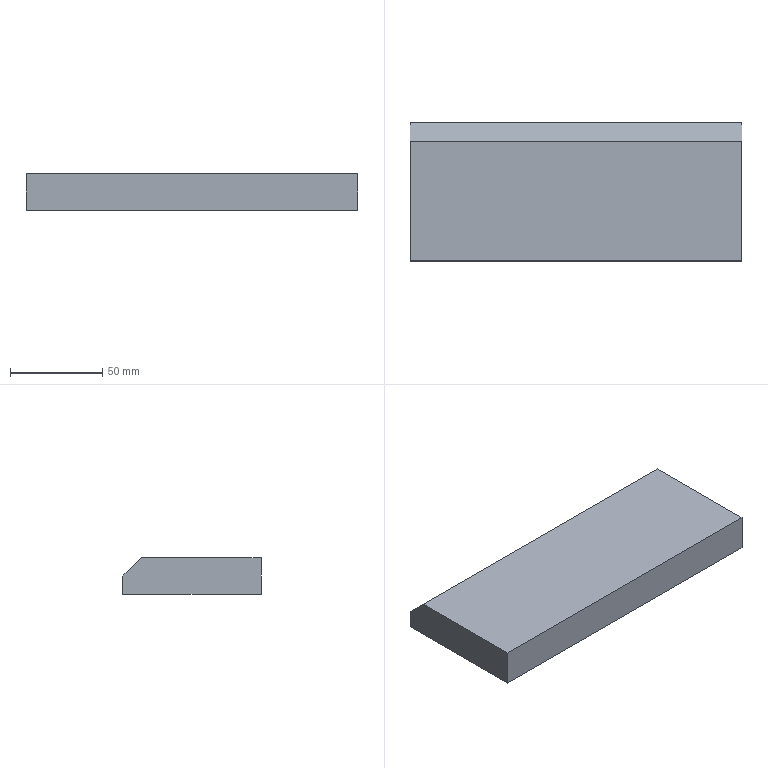Part | SolidWorks | features Chamfer 1, Extrusion 1 | 1 solid | 7 faces | box 180 x 75 x 20 mm | volume 261000 mm3 | plane 7
STEP:
#1=CARTESIAN_POINT('',(-90.,65.,20.));
#2=VERTEX_POINT('',#1);
#3=CARTESIAN_POINT('',(-90.,0.,20.));
#4=VERTEX_POINT('',#3);
#5=CARTESIAN_POINT('',(-90.,75.,20.));
#6=DIRECTION('',(0.,-1.,0.));
#7=VECTOR('',#6,1000.);
#8=LINE('',#5,#7);
#9=EDGE_CURVE('',#2,#4,#8,.T.);
#10=ORIENTED_EDGE('',*,*,#9,.F.);
#11=CARTESIAN_POINT('',(-90.,75.,10.));
#12=VERTEX_POINT('',#11);
#13=CARTESIAN_POINT('',(-90.,65.,20.));
#14=DIRECTION('',(0.,0.7071,-0.7071));
#15=VECTOR('',#14,1000.);
#16=LINE('',#13,#15);
#17=EDGE_CURVE('',#2,#12,#16,.T.);
#18=ORIENTED_EDGE('',*,*,#17,.T.);
#19=CARTESIAN_POINT('',(-90.,75.,0.));
#20=VERTEX_POINT('',#19);
#21=CARTESIAN_POINT('',(-90.,75.,20.));
#22=DIRECTION('',(0.,0.,-1.));
#23=VECTOR('',#22,1000.);
#24=LINE('',#21,#23);
#25=EDGE_CURVE('',#12,#20,#24,.T.);
#26=ORIENTED_EDGE('',*,*,#25,.T.);
#27=CARTESIAN_POINT('',(-90.,0.,0.));
#28=VERTEX_POINT('',#27);
#29=CARTESIAN_POINT('',(-90.,75.,0.));
#30=DIRECTION('',(0.,-1.,0.));
#31=VECTOR('',#30,1000.);
#32=LINE('',#29,#31);
#33=EDGE_CURVE('',#20,#28,#32,.T.);
#34=ORIENTED_EDGE('',*,*,#33,.T.);
#35=CARTESIAN_POINT('',(-90.,0.,20.));
#36=DIRECTION('',(0.,0.,-1.));
#37=VECTOR('',#36,1000.);
#38=LINE('',#35,#37);
#39=EDGE_CURVE('',#4,#28,#38,.T.);
#40=ORIENTED_EDGE('',*,*,#39,.F.);
#41=EDGE_LOOP('',(#10,#18,#26,#34,#40));
#42=FACE_OUTER_BOUND('',#41,.T.);
#43=CARTESIAN_POINT('',(-90.,75.,20.));
#44=DIRECTION('',(1.,0.,0.));
#45=DIRECTION('',(0.,0.,-1.));
#46=AXIS2_PLACEMENT_3D('',#43,#44,#45);
#47=PLANE('',#46);
#48=ADVANCED_FACE('',(#42),#47,.F.);
#49=CARTESIAN_POINT('',(90.,0.,0.));
#50=VERTEX_POINT('',#49);
#51=CARTESIAN_POINT('',(-90.,0.,0.));
#52=DIRECTION('',(1.,0.,0.));
#53=VECTOR('',#52,1000.);
#54=LINE('',#51,#53);
#55=EDGE_CURVE('',#28,#50,#54,.T.);
#56=ORIENTED_EDGE('',*,*,#55,.T.);
#57=CARTESIAN_POINT('',(90.,0.,20.));
#58=VERTEX_POINT('',#57);
#59=CARTESIAN_POINT('',(90.,0.,20.));
#60=DIRECTION('',(0.,0.,-1.));
#61=VECTOR('',#60,1000.);
#62=LINE('',#59,#61);
#63=EDGE_CURVE('',#58,#50,#62,.T.);
#64=ORIENTED_EDGE('',*,*,#63,.F.);
#65=CARTESIAN_POINT('',(-90.,0.,20.));
#66=DIRECTION('',(1.,0.,0.));
#67=VECTOR('',#66,1000.);
#68=LINE('',#65,#67);
#69=EDGE_CURVE('',#4,#58,#68,.T.);
#70=ORIENTED_EDGE('',*,*,#69,.F.);
#71=ORIENTED_EDGE('',*,*,#39,.T.);
#72=EDGE_LOOP('',(#56,#64,#70,#71));
#73=FACE_OUTER_BOUND('',#72,.T.);
#74=CARTESIAN_POINT('',(-90.,0.,20.));
#75=DIRECTION('',(0.,1.,0.));
#76=DIRECTION('',(-1.,0.,0.));
#77=AXIS2_PLACEMENT_3D('',#74,#75,#76);
#78=PLANE('',#77);
#79=ADVANCED_FACE('',(#73),#78,.F.);
#80=CARTESIAN_POINT('',(90.,75.,10.));
#81=VERTEX_POINT('',#80);
#82=CARTESIAN_POINT('',(90.,75.,0.));
#83=VERTEX_POINT('',#82);
#84=CARTESIAN_POINT('',(90.,75.,20.));
#85=DIRECTION('',(0.,0.,-1.));
#86=VECTOR('',#85,1000.);
#87=LINE('',#84,#86);
#88=EDGE_CURVE('',#81,#83,#87,.T.);
#89=ORIENTED_EDGE('',*,*,#88,.F.);
#90=CARTESIAN_POINT('',(90.,65.,20.));
#91=VERTEX_POINT('',#90);
#92=CARTESIAN_POINT('',(90.,65.,20.));
#93=DIRECTION('',(0.,-0.7071,0.7071));
#94=VECTOR('',#93,1000.);
#95=LINE('',#92,#94);
#96=EDGE_CURVE('',#81,#91,#95,.T.);
#97=ORIENTED_EDGE('',*,*,#96,.T.);
#98=CARTESIAN_POINT('',(90.,0.,20.));
#99=DIRECTION('',(0.,1.,0.));
#100=VECTOR('',#99,1000.);
#101=LINE('',#98,#100);
#102=EDGE_CURVE('',#58,#91,#101,.T.);
#103=ORIENTED_EDGE('',*,*,#102,.F.);
#104=ORIENTED_EDGE('',*,*,#63,.T.);
#105=CARTESIAN_POINT('',(90.,0.,0.));
#106=DIRECTION('',(0.,1.,0.));
#107=VECTOR('',#106,1000.);
#108=LINE('',#105,#107);
#109=EDGE_CURVE('',#50,#83,#108,.T.);
#110=ORIENTED_EDGE('',*,*,#109,.T.);
#111=EDGE_LOOP('',(#89,#97,#103,#104,#110));
#112=FACE_OUTER_BOUND('',#111,.T.);
#113=CARTESIAN_POINT('',(90.,0.,20.));
#114=DIRECTION('',(-1.,0.,0.));
#115=DIRECTION('',(0.,-1.,0.));
#116=AXIS2_PLACEMENT_3D('',#113,#114,#115);
#117=PLANE('',#116);
#118=ADVANCED_FACE('',(#112),#117,.F.);
#119=ORIENTED_EDGE('',*,*,#25,.F.);
#120=CARTESIAN_POINT('',(90.,75.,10.));
#121=DIRECTION('',(1.,0.,0.));
#122=VECTOR('',#121,1000.);
#123=LINE('',#120,#122);
#124=EDGE_CURVE('',#12,#81,#123,.T.);
#125=ORIENTED_EDGE('',*,*,#124,.T.);
#126=ORIENTED_EDGE('',*,*,#88,.T.);
#127=CARTESIAN_POINT('',(90.,75.,0.));
#128=DIRECTION('',(-1.,0.,0.));
#129=VECTOR('',#128,1000.);
#130=LINE('',#127,#129);
#131=EDGE_CURVE('',#83,#20,#130,.T.);
#132=ORIENTED_EDGE('',*,*,#131,.T.);
#133=EDGE_LOOP('',(#119,#125,#126,#132));
#134=FACE_OUTER_BOUND('',#133,.T.);
#135=CARTESIAN_POINT('',(90.,75.,20.));
#136=DIRECTION('',(0.,-1.,0.));
#137=DIRECTION('',(1.,0.,0.));
#138=AXIS2_PLACEMENT_3D('',#135,#136,#137);
#139=PLANE('',#138);
#140=ADVANCED_FACE('',(#134),#139,.F.);
#141=ORIENTED_EDGE('',*,*,#102,.T.);
#142=CARTESIAN_POINT('',(-90.,65.,20.));
#143=DIRECTION('',(-1.,0.,0.));
#144=VECTOR('',#143,1000.);
#145=LINE('',#142,#144);
#146=EDGE_CURVE('',#91,#2,#145,.T.);
#147=ORIENTED_EDGE('',*,*,#146,.T.);
#148=ORIENTED_EDGE('',*,*,#9,.T.);
#149=ORIENTED_EDGE('',*,*,#69,.T.);
#150=EDGE_LOOP('',(#141,#147,#148,#149));
#151=FACE_OUTER_BOUND('',#150,.T.);
#152=CARTESIAN_POINT('',(0.,0.,20.));
#153=DIRECTION('',(0.,0.,1.));
#154=DIRECTION('',(1.,0.,0.));
#155=AXIS2_PLACEMENT_3D('',#152,#153,#154);
#156=PLANE('',#155);
#157=ADVANCED_FACE('',(#151),#156,.T.);
#158=ORIENTED_EDGE('',*,*,#33,.F.);
#159=ORIENTED_EDGE('',*,*,#131,.F.);
#160=ORIENTED_EDGE('',*,*,#109,.F.);
#161=ORIENTED_EDGE('',*,*,#55,.F.);
#162=EDGE_LOOP('',(#158,#159,#160,#161));
#163=FACE_OUTER_BOUND('',#162,.T.);
#164=CARTESIAN_POINT('',(0.,0.,0.));
#165=DIRECTION('',(0.,0.,1.));
#166=DIRECTION('',(1.,0.,0.));
#167=AXIS2_PLACEMENT_3D('',#164,#165,#166);
#168=PLANE('',#167);
#169=ADVANCED_FACE('',(#163),#168,.F.);
#170=ORIENTED_EDGE('',*,*,#96,.F.);
#171=ORIENTED_EDGE('',*,*,#124,.F.);
#172=ORIENTED_EDGE('',*,*,#17,.F.);
#173=ORIENTED_EDGE('',*,*,#146,.F.);
#174=EDGE_LOOP('',(#170,#171,#172,#173));
#175=FACE_OUTER_BOUND('',#174,.T.);
#176=CARTESIAN_POINT('',(0.,65.,20.));
#177=DIRECTION('',(0.,0.7071,0.7071));
#178=DIRECTION('',(1.,0.,0.));
#179=AXIS2_PLACEMENT_3D('',#176,#177,#178);
#180=PLANE('',#179);
#181=ADVANCED_FACE('',(#175),#180,.T.);
#182=CLOSED_SHELL('',(#48,#79,#118,#140,#157,#169,#181));
#183=MANIFOLD_SOLID_BREP('',#182);
#184=CARTESIAN_POINT('',(0.,0.,0.));
#185=DIRECTION('',(0.,0.,1.));
#186=DIRECTION('',(1.,0.,0.));
#187=AXIS2_PLACEMENT_3D('',#184,#185,#186);
#188=(LENGTH_UNIT()NAMED_UNIT(*)SI_UNIT(.MILLI.,.METRE.));
#189=UNCERTAINTY_MEASURE_WITH_UNIT(LENGTH_MEASURE(0.00001),#188,'','');
#190=(NAMED_UNIT(*)PLANE_ANGLE_UNIT()SI_UNIT($,.RADIAN.));
#191=(NAMED_UNIT(*)SI_UNIT($,.STERADIAN.)SOLID_ANGLE_UNIT());
#192=(GEOMETRIC_REPRESENTATION_CONTEXT(3)GLOBAL_UNCERTAINTY_ASSIGNED_CONTEXT((#189))GLOBAL_UNIT_ASSIGNED_CONTEXT((#188,#190,#191))REPRESENTATION_CONTEXT('',''));
#193=ADVANCED_BREP_SHAPE_REPRESENTATION('',(#183,#187),#192);